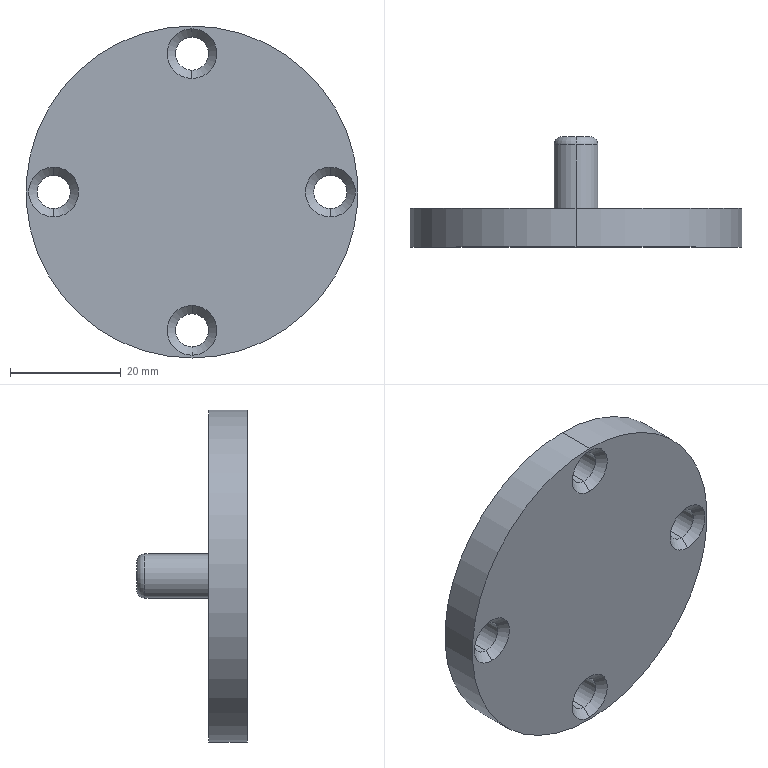Part | SolidWorks | features ICE 2, Extrusion 1, Fillet 1, HoleWzd 1 | 1 solid | 28 faces | box 60 x 20 x 60 mm | volume 17734 mm3 | cylinder 14 | cone 8 | plane 4 | torus 2 | commonest cylinder face diameters 6 x8 8 x2 40 x2 60 x2
STEP:
#1=CARTESIAN_POINT('',(0.,18.5,-4.));
#2=VERTEX_POINT('',#1);
#3=CARTESIAN_POINT('',(0.,18.5,4.));
#4=VERTEX_POINT('',#3);
#5=CARTESIAN_POINT('',(0.,18.5,0.));
#6=DIRECTION('',(0.,-1.,0.));
#7=DIRECTION('',(0.,0.,1.));
#8=AXIS2_PLACEMENT_3D('',#5,#6,#7);
#9=CIRCLE('',#8,4.);
#10=EDGE_CURVE('',#2,#4,#9,.T.);
#11=ORIENTED_EDGE('',*,*,#10,.F.);
#12=CARTESIAN_POINT('',(0.,20.,-2.5));
#13=VERTEX_POINT('',#12);
#14=CARTESIAN_POINT('',(0.,18.5,-2.5));
#15=DIRECTION('',(1.,0.,0.));
#16=DIRECTION('',(0.,0.,-1.));
#17=AXIS2_PLACEMENT_3D('',#14,#15,#16);
#18=CIRCLE('',#17,1.5);
#19=EDGE_CURVE('',#2,#13,#18,.T.);
#20=ORIENTED_EDGE('',*,*,#19,.T.);
#21=CARTESIAN_POINT('',(0.,20.,2.5));
#22=VERTEX_POINT('',#21);
#23=CARTESIAN_POINT('',(0.,20.,0.));
#24=DIRECTION('',(0.,1.,0.));
#25=DIRECTION('',(0.,0.,1.));
#26=AXIS2_PLACEMENT_3D('',#23,#24,#25);
#27=CIRCLE('',#26,2.5);
#28=EDGE_CURVE('',#22,#13,#27,.T.);
#29=ORIENTED_EDGE('',*,*,#28,.F.);
#30=CARTESIAN_POINT('',(0.,18.5,2.5));
#31=DIRECTION('',(-1.,0.,0.));
#32=DIRECTION('',(0.,0.,1.));
#33=AXIS2_PLACEMENT_3D('',#30,#31,#32);
#34=CIRCLE('',#33,1.5);
#35=EDGE_CURVE('',#4,#22,#34,.T.);
#36=ORIENTED_EDGE('',*,*,#35,.F.);
#37=EDGE_LOOP('',(#11,#20,#29,#36));
#38=FACE_OUTER_BOUND('',#37,.T.);
#39=CARTESIAN_POINT('',(0.,18.5,0.));
#40=DIRECTION('',(0.,1.,0.));
#41=DIRECTION('',(0.,0.,1.));
#42=AXIS2_PLACEMENT_3D('',#39,#40,#41);
#43=TOROIDAL_SURFACE('',#42,2.5,1.5);
#44=ADVANCED_FACE('',(#38),#43,.T.);
#45=CARTESIAN_POINT('',(0.,1.5,-22.));
#46=VERTEX_POINT('',#45);
#47=CARTESIAN_POINT('',(0.,1.5,-28.));
#48=VERTEX_POINT('',#47);
#49=CARTESIAN_POINT('',(0.,1.5,-25.));
#50=DIRECTION('',(0.,-1.,0.));
#51=DIRECTION('',(0.,0.,-1.));
#52=AXIS2_PLACEMENT_3D('',#49,#50,#51);
#53=CIRCLE('',#52,3.);
#54=EDGE_CURVE('',#46,#48,#53,.T.);
#55=ORIENTED_EDGE('',*,*,#54,.F.);
#56=CARTESIAN_POINT('',(0.,0.,-20.5));
#57=VERTEX_POINT('',#56);
#58=CARTESIAN_POINT('',(0.,0.,-20.5));
#59=DIRECTION('',(0.,-0.7071,0.7071));
#60=VECTOR('',#59,1000.);
#61=LINE('',#58,#60);
#62=EDGE_CURVE('',#46,#57,#61,.T.);
#63=ORIENTED_EDGE('',*,*,#62,.T.);
#64=CARTESIAN_POINT('',(0.,0.,-29.5));
#65=VERTEX_POINT('',#64);
#66=CARTESIAN_POINT('',(0.,0.,-25.));
#67=DIRECTION('',(0.,-1.,0.));
#68=DIRECTION('',(0.,0.,-1.));
#69=AXIS2_PLACEMENT_3D('',#66,#67,#68);
#70=CIRCLE('',#69,4.5);
#71=EDGE_CURVE('',#57,#65,#70,.T.);
#72=ORIENTED_EDGE('',*,*,#71,.T.);
#73=CARTESIAN_POINT('',(0.,0.,-29.5));
#74=DIRECTION('',(0.,-0.7071,-0.7071));
#75=VECTOR('',#74,1000.);
#76=LINE('',#73,#75);
#77=EDGE_CURVE('',#48,#65,#76,.T.);
#78=ORIENTED_EDGE('',*,*,#77,.F.);
#79=EDGE_LOOP('',(#55,#63,#72,#78));
#80=FACE_OUTER_BOUND('',#79,.T.);
#81=CARTESIAN_POINT('',(0.,0.,-25.));
#82=DIRECTION('',(0.,-1.,0.));
#83=DIRECTION('',(0.,0.,-1.));
#84=AXIS2_PLACEMENT_3D('',#81,#82,#83);
#85=CONICAL_SURFACE('',#84,4.5,0.7854);
#86=ADVANCED_FACE('',(#80),#85,.F.);
#87=CARTESIAN_POINT('',(0.,7.,-28.));
#88=VERTEX_POINT('',#87);
#89=CARTESIAN_POINT('',(0.,7.,-22.));
#90=VERTEX_POINT('',#89);
#91=CARTESIAN_POINT('',(0.,7.,-25.));
#92=DIRECTION('',(0.,1.,0.));
#93=DIRECTION('',(0.,0.,1.));
#94=AXIS2_PLACEMENT_3D('',#91,#92,#93);
#95=CIRCLE('',#94,3.);
#96=EDGE_CURVE('',#88,#90,#95,.T.);
#97=ORIENTED_EDGE('',*,*,#96,.T.);
#98=CARTESIAN_POINT('',(0.,0.,-22.));
#99=DIRECTION('',(0.,-1.,0.));
#100=VECTOR('',#99,1000.);
#101=LINE('',#98,#100);
#102=EDGE_CURVE('',#90,#46,#101,.T.);
#103=ORIENTED_EDGE('',*,*,#102,.T.);
#104=ORIENTED_EDGE('',*,*,#54,.T.);
#105=CARTESIAN_POINT('',(0.,0.,-28.));
#106=DIRECTION('',(0.,-1.,0.));
#107=VECTOR('',#106,1000.);
#108=LINE('',#105,#107);
#109=EDGE_CURVE('',#88,#48,#108,.T.);
#110=ORIENTED_EDGE('',*,*,#109,.F.);
#111=EDGE_LOOP('',(#97,#103,#104,#110));
#112=FACE_OUTER_BOUND('',#111,.T.);
#113=CARTESIAN_POINT('',(0.,0.,-25.));
#114=DIRECTION('',(0.,-1.,0.));
#115=DIRECTION('',(0.,0.,-1.));
#116=AXIS2_PLACEMENT_3D('',#113,#114,#115);
#117=CYLINDRICAL_SURFACE('',#116,3.);
#118=ADVANCED_FACE('',(#112),#117,.F.);
#119=CARTESIAN_POINT('',(-25.,1.5,3.));
#120=VERTEX_POINT('',#119);
#121=CARTESIAN_POINT('',(-25.,1.5,-3.));
#122=VERTEX_POINT('',#121);
#123=CARTESIAN_POINT('',(-25.,1.5,0.));
#124=DIRECTION('',(0.,-1.,0.));
#125=DIRECTION('',(0.,0.,-1.));
#126=AXIS2_PLACEMENT_3D('',#123,#124,#125);
#127=CIRCLE('',#126,3.);
#128=EDGE_CURVE('',#120,#122,#127,.T.);
#129=ORIENTED_EDGE('',*,*,#128,.F.);
#130=CARTESIAN_POINT('',(-25.,0.,4.5));
#131=VERTEX_POINT('',#130);
#132=CARTESIAN_POINT('',(-25.,0.,4.5));
#133=DIRECTION('',(0.,-0.7071,0.7071));
#134=VECTOR('',#133,1000.);
#135=LINE('',#132,#134);
#136=EDGE_CURVE('',#120,#131,#135,.T.);
#137=ORIENTED_EDGE('',*,*,#136,.T.);
#138=CARTESIAN_POINT('',(-25.,0.,-4.5));
#139=VERTEX_POINT('',#138);
#140=CARTESIAN_POINT('',(-25.,0.,0.));
#141=DIRECTION('',(0.,-1.,0.));
#142=DIRECTION('',(0.,0.,-1.));
#143=AXIS2_PLACEMENT_3D('',#140,#141,#142);
#144=CIRCLE('',#143,4.5);
#145=EDGE_CURVE('',#131,#139,#144,.T.);
#146=ORIENTED_EDGE('',*,*,#145,.T.);
#147=CARTESIAN_POINT('',(-25.,0.,-4.5));
#148=DIRECTION('',(0.,-0.7071,-0.7071));
#149=VECTOR('',#148,1000.);
#150=LINE('',#147,#149);
#151=EDGE_CURVE('',#122,#139,#150,.T.);
#152=ORIENTED_EDGE('',*,*,#151,.F.);
#153=EDGE_LOOP('',(#129,#137,#146,#152));
#154=FACE_OUTER_BOUND('',#153,.T.);
#155=CARTESIAN_POINT('',(-25.,0.,0.));
#156=DIRECTION('',(0.,-1.,0.));
#157=DIRECTION('',(0.,0.,-1.));
#158=AXIS2_PLACEMENT_3D('',#155,#156,#157);
#159=CONICAL_SURFACE('',#158,4.5,0.7854);
#160=ADVANCED_FACE('',(#154),#159,.F.);
#161=CARTESIAN_POINT('',(-25.,7.,-3.));
#162=VERTEX_POINT('',#161);
#163=CARTESIAN_POINT('',(-25.,7.,3.));
#164=VERTEX_POINT('',#163);
#165=CARTESIAN_POINT('',(-25.,7.,0.));
#166=DIRECTION('',(0.,1.,0.));
#167=DIRECTION('',(0.,0.,1.));
#168=AXIS2_PLACEMENT_3D('',#165,#166,#167);
#169=CIRCLE('',#168,3.);
#170=EDGE_CURVE('',#162,#164,#169,.T.);
#171=ORIENTED_EDGE('',*,*,#170,.T.);
#172=CARTESIAN_POINT('',(-25.,0.,3.));
#173=DIRECTION('',(0.,-1.,0.));
#174=VECTOR('',#173,1000.);
#175=LINE('',#172,#174);
#176=EDGE_CURVE('',#164,#120,#175,.T.);
#177=ORIENTED_EDGE('',*,*,#176,.T.);
#178=ORIENTED_EDGE('',*,*,#128,.T.);
#179=CARTESIAN_POINT('',(-25.,0.,-3.));
#180=DIRECTION('',(0.,-1.,0.));
#181=VECTOR('',#180,1000.);
#182=LINE('',#179,#181);
#183=EDGE_CURVE('',#162,#122,#182,.T.);
#184=ORIENTED_EDGE('',*,*,#183,.F.);
#185=EDGE_LOOP('',(#171,#177,#178,#184));
#186=FACE_OUTER_BOUND('',#185,.T.);
#187=CARTESIAN_POINT('',(-25.,0.,0.));
#188=DIRECTION('',(0.,-1.,0.));
#189=DIRECTION('',(0.,0.,-1.));
#190=AXIS2_PLACEMENT_3D('',#187,#188,#189);
#191=CYLINDRICAL_SURFACE('',#190,3.);
#192=ADVANCED_FACE('',(#186),#191,.F.);
#193=CARTESIAN_POINT('',(0.,1.5,28.));
#194=VERTEX_POINT('',#193);
#195=CARTESIAN_POINT('',(0.,1.5,22.));
#196=VERTEX_POINT('',#195);
#197=CARTESIAN_POINT('',(0.,1.5,25.));
#198=DIRECTION('',(0.,-1.,0.));
#199=DIRECTION('',(0.,0.,-1.));
#200=AXIS2_PLACEMENT_3D('',#197,#198,#199);
#201=CIRCLE('',#200,3.);
#202=EDGE_CURVE('',#194,#196,#201,.T.);
#203=ORIENTED_EDGE('',*,*,#202,.F.);
#204=CARTESIAN_POINT('',(0.,0.,29.5));
#205=VERTEX_POINT('',#204);
#206=CARTESIAN_POINT('',(0.,0.,29.5));
#207=DIRECTION('',(0.,-0.7071,0.7071));
#208=VECTOR('',#207,1000.);
#209=LINE('',#206,#208);
#210=EDGE_CURVE('',#194,#205,#209,.T.);
#211=ORIENTED_EDGE('',*,*,#210,.T.);
#212=CARTESIAN_POINT('',(0.,0.,20.5));
#213=VERTEX_POINT('',#212);
#214=CARTESIAN_POINT('',(0.,0.,25.));
#215=DIRECTION('',(0.,-1.,0.));
#216=DIRECTION('',(0.,0.,-1.));
#217=AXIS2_PLACEMENT_3D('',#214,#215,#216);
#218=CIRCLE('',#217,4.5);
#219=EDGE_CURVE('',#205,#213,#218,.T.);
#220=ORIENTED_EDGE('',*,*,#219,.T.);
#221=CARTESIAN_POINT('',(0.,0.,20.5));
#222=DIRECTION('',(0.,-0.7071,-0.7071));
#223=VECTOR('',#222,1000.);
#224=LINE('',#221,#223);
#225=EDGE_CURVE('',#196,#213,#224,.T.);
#226=ORIENTED_EDGE('',*,*,#225,.F.);
#227=EDGE_LOOP('',(#203,#211,#220,#226));
#228=FACE_OUTER_BOUND('',#227,.T.);
#229=CARTESIAN_POINT('',(0.,0.,25.));
#230=DIRECTION('',(0.,-1.,0.));
#231=DIRECTION('',(0.,0.,-1.));
#232=AXIS2_PLACEMENT_3D('',#229,#230,#231);
#233=CONICAL_SURFACE('',#232,4.5,0.7854);
#234=ADVANCED_FACE('',(#228),#233,.F.);
#235=CARTESIAN_POINT('',(0.,7.,22.));
#236=VERTEX_POINT('',#235);
#237=CARTESIAN_POINT('',(0.,7.,28.));
#238=VERTEX_POINT('',#237);
#239=CARTESIAN_POINT('',(0.,7.,25.));
#240=DIRECTION('',(0.,1.,0.));
#241=DIRECTION('',(0.,0.,1.));
#242=AXIS2_PLACEMENT_3D('',#239,#240,#241);
#243=CIRCLE('',#242,3.);
#244=EDGE_CURVE('',#236,#238,#243,.T.);
#245=ORIENTED_EDGE('',*,*,#244,.T.);
#246=CARTESIAN_POINT('',(0.,0.,28.));
#247=DIRECTION('',(0.,-1.,0.));
#248=VECTOR('',#247,1000.);
#249=LINE('',#246,#248);
#250=EDGE_CURVE('',#238,#194,#249,.T.);
#251=ORIENTED_EDGE('',*,*,#250,.T.);
#252=ORIENTED_EDGE('',*,*,#202,.T.);
#253=CARTESIAN_POINT('',(0.,0.,22.));
#254=DIRECTION('',(0.,-1.,0.));
#255=VECTOR('',#254,1000.);
#256=LINE('',#253,#255);
#257=EDGE_CURVE('',#236,#196,#256,.T.);
#258=ORIENTED_EDGE('',*,*,#257,.F.);
#259=EDGE_LOOP('',(#245,#251,#252,#258));
#260=FACE_OUTER_BOUND('',#259,.T.);
#261=CARTESIAN_POINT('',(0.,0.,25.));
#262=DIRECTION('',(0.,-1.,0.));
#263=DIRECTION('',(0.,0.,-1.));
#264=AXIS2_PLACEMENT_3D('',#261,#262,#263);
#265=CYLINDRICAL_SURFACE('',#264,3.);
#266=ADVANCED_FACE('',(#260),#265,.F.);
#267=CARTESIAN_POINT('',(25.,1.5,3.));
#268=VERTEX_POINT('',#267);
#269=CARTESIAN_POINT('',(25.,1.5,-3.));
#270=VERTEX_POINT('',#269);
#271=CARTESIAN_POINT('',(25.,1.5,0.));
#272=DIRECTION('',(0.,-1.,0.));
#273=DIRECTION('',(0.,0.,-1.));
#274=AXIS2_PLACEMENT_3D('',#271,#272,#273);
#275=CIRCLE('',#274,3.);
#276=EDGE_CURVE('',#268,#270,#275,.T.);
#277=ORIENTED_EDGE('',*,*,#276,.F.);
#278=CARTESIAN_POINT('',(25.,0.,4.5));
#279=VERTEX_POINT('',#278);
#280=CARTESIAN_POINT('',(25.,0.,4.5));
#281=DIRECTION('',(0.,-0.7071,0.7071));
#282=VECTOR('',#281,1000.);
#283=LINE('',#280,#282);
#284=EDGE_CURVE('',#268,#279,#283,.T.);
#285=ORIENTED_EDGE('',*,*,#284,.T.);
#286=CARTESIAN_POINT('',(25.,0.,-4.5));
#287=VERTEX_POINT('',#286);
#288=CARTESIAN_POINT('',(25.,0.,0.));
#289=DIRECTION('',(0.,-1.,0.));
#290=DIRECTION('',(0.,0.,-1.));
#291=AXIS2_PLACEMENT_3D('',#288,#289,#290);
#292=CIRCLE('',#291,4.5);
#293=EDGE_CURVE('',#279,#287,#292,.T.);
#294=ORIENTED_EDGE('',*,*,#293,.T.);
#295=CARTESIAN_POINT('',(25.,0.,-4.5));
#296=DIRECTION('',(0.,-0.7071,-0.7071));
#297=VECTOR('',#296,1000.);
#298=LINE('',#295,#297);
#299=EDGE_CURVE('',#270,#287,#298,.T.);
#300=ORIENTED_EDGE('',*,*,#299,.F.);
#301=EDGE_LOOP('',(#277,#285,#294,#300));
#302=FACE_OUTER_BOUND('',#301,.T.);
#303=CARTESIAN_POINT('',(25.,0.,0.));
#304=DIRECTION('',(0.,-1.,0.));
#305=DIRECTION('',(0.,0.,-1.));
#306=AXIS2_PLACEMENT_3D('',#303,#304,#305);
#307=CONICAL_SURFACE('',#306,4.5,0.7854);
#308=ADVANCED_FACE('',(#302),#307,.F.);
#309=CARTESIAN_POINT('',(25.,7.,-3.));
#310=VERTEX_POINT('',#309);
#311=CARTESIAN_POINT('',(25.,7.,3.));
#312=VERTEX_POINT('',#311);
#313=CARTESIAN_POINT('',(25.,7.,0.));
#314=DIRECTION('',(0.,1.,0.));
#315=DIRECTION('',(0.,0.,1.));
#316=AXIS2_PLACEMENT_3D('',#313,#314,#315);
#317=CIRCLE('',#316,3.);
#318=EDGE_CURVE('',#310,#312,#317,.T.);
#319=ORIENTED_EDGE('',*,*,#318,.T.);
#320=CARTESIAN_POINT('',(25.,0.,3.));
#321=DIRECTION('',(0.,-1.,0.));
#322=VECTOR('',#321,1000.);
#323=LINE('',#320,#322);
#324=EDGE_CURVE('',#312,#268,#323,.T.);
#325=ORIENTED_EDGE('',*,*,#324,.T.);
#326=ORIENTED_EDGE('',*,*,#276,.T.);
#327=CARTESIAN_POINT('',(25.,0.,-3.));
#328=DIRECTION('',(0.,-1.,0.));
#329=VECTOR('',#328,1000.);
#330=LINE('',#327,#329);
#331=EDGE_CURVE('',#310,#270,#330,.T.);
#332=ORIENTED_EDGE('',*,*,#331,.F.);
#333=EDGE_LOOP('',(#319,#325,#326,#332));
#334=FACE_OUTER_BOUND('',#333,.T.);
#335=CARTESIAN_POINT('',(25.,0.,0.));
#336=DIRECTION('',(0.,-1.,0.));
#337=DIRECTION('',(0.,0.,-1.));
#338=AXIS2_PLACEMENT_3D('',#335,#336,#337);
#339=CYLINDRICAL_SURFACE('',#338,3.);
#340=ADVANCED_FACE('',(#334),#339,.F.);
#341=ORIENTED_EDGE('',*,*,#10,.T.);
#342=CARTESIAN_POINT('',(0.,5.5,4.));
#343=VERTEX_POINT('',#342);
#344=CARTESIAN_POINT('',(0.,20.,4.));
#345=DIRECTION('',(0.,-1.,0.));
#346=VECTOR('',#345,1000.);
#347=LINE('',#344,#346);
#348=EDGE_CURVE('',#4,#343,#347,.T.);
#349=ORIENTED_EDGE('',*,*,#348,.T.);
#350=CARTESIAN_POINT('',(0.,5.5,-4.));
#351=VERTEX_POINT('',#350);
#352=CARTESIAN_POINT('',(0.,5.5,0.));
#353=DIRECTION('',(0.,1.,0.));
#354=DIRECTION('',(0.,0.,1.));
#355=AXIS2_PLACEMENT_3D('',#352,#353,#354);
#356=CIRCLE('',#355,4.);
#357=EDGE_CURVE('',#343,#351,#356,.T.);
#358=ORIENTED_EDGE('',*,*,#357,.T.);
#359=CARTESIAN_POINT('',(0.,20.,-4.));
#360=DIRECTION('',(0.,-1.,0.));
#361=VECTOR('',#360,1000.);
#362=LINE('',#359,#361);
#363=EDGE_CURVE('',#2,#351,#362,.T.);
#364=ORIENTED_EDGE('',*,*,#363,.F.);
#365=EDGE_LOOP('',(#341,#349,#358,#364));
#366=FACE_OUTER_BOUND('',#365,.T.);
#367=CARTESIAN_POINT('',(0.,20.,0.));
#368=DIRECTION('',(0.,-1.,0.));
#369=DIRECTION('',(0.,0.,-1.));
#370=AXIS2_PLACEMENT_3D('',#367,#368,#369);
#371=CYLINDRICAL_SURFACE('',#370,4.);
#372=ADVANCED_FACE('',(#366),#371,.T.);
#373=CARTESIAN_POINT('',(0.,5.5,-20.));
#374=VERTEX_POINT('',#373);
#375=CARTESIAN_POINT('',(0.,5.5,20.));
#376=VERTEX_POINT('',#375);
#377=CARTESIAN_POINT('',(0.,5.5,0.));
#378=DIRECTION('',(0.,1.,0.));
#379=DIRECTION('',(0.,0.,1.));
#380=AXIS2_PLACEMENT_3D('',#377,#378,#379);
#381=CIRCLE('',#380,20.);
#382=EDGE_CURVE('',#374,#376,#381,.T.);
#383=ORIENTED_EDGE('',*,*,#382,.F.);
#384=CARTESIAN_POINT('',(0.,7.,-20.));
#385=VERTEX_POINT('',#384);
#386=CARTESIAN_POINT('',(0.,5.5,-20.));
#387=DIRECTION('',(0.,1.,0.));
#388=VECTOR('',#387,1000.);
#389=LINE('',#386,#388);
#390=EDGE_CURVE('',#374,#385,#389,.T.);
#391=ORIENTED_EDGE('',*,*,#390,.T.);
#392=CARTESIAN_POINT('',(0.,7.,20.));
#393=VERTEX_POINT('',#392);
#394=CARTESIAN_POINT('',(0.,7.,0.));
#395=DIRECTION('',(0.,1.,0.));
#396=DIRECTION('',(0.,0.,1.));
#397=AXIS2_PLACEMENT_3D('',#394,#395,#396);
#398=CIRCLE('',#397,20.);
#399=EDGE_CURVE('',#385,#393,#398,.T.);
#400=ORIENTED_EDGE('',*,*,#399,.T.);
#401=CARTESIAN_POINT('',(0.,5.5,20.));
#402=DIRECTION('',(0.,1.,0.));
#403=VECTOR('',#402,1000.);
#404=LINE('',#401,#403);
#405=EDGE_CURVE('',#376,#393,#404,.T.);
#406=ORIENTED_EDGE('',*,*,#405,.F.);
#407=EDGE_LOOP('',(#383,#391,#400,#406));
#408=FACE_OUTER_BOUND('',#407,.T.);
#409=CARTESIAN_POINT('',(0.,5.5,0.));
#410=DIRECTION('',(0.,1.,0.));
#411=DIRECTION('',(0.,0.,1.));
#412=AXIS2_PLACEMENT_3D('',#409,#410,#411);
#413=CYLINDRICAL_SURFACE('',#412,20.);
#414=ADVANCED_FACE('',(#408),#413,.F.);
#415=CARTESIAN_POINT('',(0.,7.,30.));
#416=VERTEX_POINT('',#415);
#417=CARTESIAN_POINT('',(0.,7.,-30.));
#418=VERTEX_POINT('',#417);
#419=CARTESIAN_POINT('',(0.,7.,0.));
#420=DIRECTION('',(0.,1.,0.));
#421=DIRECTION('',(0.,0.,1.));
#422=AXIS2_PLACEMENT_3D('',#419,#420,#421);
#423=CIRCLE('',#422,30.);
#424=EDGE_CURVE('',#416,#418,#423,.T.);
#425=ORIENTED_EDGE('',*,*,#424,.F.);
#426=CARTESIAN_POINT('',(0.,0.,30.));
#427=VERTEX_POINT('',#426);
#428=CARTESIAN_POINT('',(0.,7.,30.));
#429=DIRECTION('',(0.,-1.,0.));
#430=VECTOR('',#429,1000.);
#431=LINE('',#428,#430);
#432=EDGE_CURVE('',#416,#427,#431,.T.);
#433=ORIENTED_EDGE('',*,*,#432,.T.);
#434=CARTESIAN_POINT('',(0.,0.,-30.));
#435=VERTEX_POINT('',#434);
#436=CARTESIAN_POINT('',(0.,0.,0.));
#437=DIRECTION('',(0.,1.,0.));
#438=DIRECTION('',(0.,0.,1.));
#439=AXIS2_PLACEMENT_3D('',#436,#437,#438);
#440=CIRCLE('',#439,30.);
#441=EDGE_CURVE('',#427,#435,#440,.T.);
#442=ORIENTED_EDGE('',*,*,#441,.T.);
#443=CARTESIAN_POINT('',(0.,7.,-30.));
#444=DIRECTION('',(0.,-1.,0.));
#445=VECTOR('',#444,1000.);
#446=LINE('',#443,#445);
#447=EDGE_CURVE('',#418,#435,#446,.T.);
#448=ORIENTED_EDGE('',*,*,#447,.F.);
#449=EDGE_LOOP('',(#425,#433,#442,#448));
#450=FACE_OUTER_BOUND('',#449,.T.);
#451=CARTESIAN_POINT('',(0.,7.,0.));
#452=DIRECTION('',(0.,-1.,0.));
#453=DIRECTION('',(0.,0.,-1.));
#454=AXIS2_PLACEMENT_3D('',#451,#452,#453);
#455=CYLINDRICAL_SURFACE('',#454,30.);
#456=ADVANCED_FACE('',(#450),#455,.T.);
#457=ORIENTED_EDGE('',*,*,#432,.F.);
#458=CARTESIAN_POINT('',(0.,7.,0.));
#459=DIRECTION('',(0.,1.,0.));
#460=DIRECTION('',(0.,0.,1.));
#461=AXIS2_PLACEMENT_3D('',#458,#459,#460);
#462=CIRCLE('',#461,30.);
#463=EDGE_CURVE('',#418,#416,#462,.T.);
#464=ORIENTED_EDGE('',*,*,#463,.F.);
#465=ORIENTED_EDGE('',*,*,#447,.T.);
#466=CARTESIAN_POINT('',(0.,0.,0.));
#467=DIRECTION('',(0.,1.,0.));
#468=DIRECTION('',(0.,0.,1.));
#469=AXIS2_PLACEMENT_3D('',#466,#467,#468);
#470=CIRCLE('',#469,30.);
#471=EDGE_CURVE('',#435,#427,#470,.T.);
#472=ORIENTED_EDGE('',*,*,#471,.T.);
#473=EDGE_LOOP('',(#457,#464,#465,#472));
#474=FACE_OUTER_BOUND('',#473,.T.);
#475=CARTESIAN_POINT('',(0.,7.,0.));
#476=DIRECTION('',(0.,-1.,0.));
#477=DIRECTION('',(0.,0.,-1.));
#478=AXIS2_PLACEMENT_3D('',#475,#476,#477);
#479=CYLINDRICAL_SURFACE('',#478,30.);
#480=ADVANCED_FACE('',(#474),#479,.T.);
#481=ORIENTED_EDGE('',*,*,#96,.F.);
#482=CARTESIAN_POINT('',(0.,7.,-25.));
#483=DIRECTION('',(0.,1.,0.));
#484=DIRECTION('',(0.,0.,1.));
#485=AXIS2_PLACEMENT_3D('',#482,#483,#484);
#486=CIRCLE('',#485,3.);
#487=EDGE_CURVE('',#90,#88,#486,.T.);
#488=ORIENTED_EDGE('',*,*,#487,.F.);
#489=EDGE_LOOP('',(#481,#488));
#490=FACE_BOUND('',#489,.T.);
#491=ORIENTED_EDGE('',*,*,#170,.F.);
#492=CARTESIAN_POINT('',(-25.,7.,0.));
#493=DIRECTION('',(0.,1.,0.));
#494=DIRECTION('',(0.,0.,1.));
#495=AXIS2_PLACEMENT_3D('',#492,#493,#494);
#496=CIRCLE('',#495,3.);
#497=EDGE_CURVE('',#164,#162,#496,.T.);
#498=ORIENTED_EDGE('',*,*,#497,.F.);
#499=EDGE_LOOP('',(#491,#498));
#500=FACE_BOUND('',#499,.T.);
#501=ORIENTED_EDGE('',*,*,#244,.F.);
#502=CARTESIAN_POINT('',(0.,7.,25.));
#503=DIRECTION('',(0.,1.,0.));
#504=DIRECTION('',(0.,0.,1.));
#505=AXIS2_PLACEMENT_3D('',#502,#503,#504);
#506=CIRCLE('',#505,3.);
#507=EDGE_CURVE('',#238,#236,#506,.T.);
#508=ORIENTED_EDGE('',*,*,#507,.F.);
#509=EDGE_LOOP('',(#501,#508));
#510=FACE_BOUND('',#509,.T.);
#511=ORIENTED_EDGE('',*,*,#318,.F.);
#512=CARTESIAN_POINT('',(25.,7.,0.));
#513=DIRECTION('',(0.,1.,0.));
#514=DIRECTION('',(0.,0.,1.));
#515=AXIS2_PLACEMENT_3D('',#512,#513,#514);
#516=CIRCLE('',#515,3.);
#517=EDGE_CURVE('',#312,#310,#516,.T.);
#518=ORIENTED_EDGE('',*,*,#517,.F.);
#519=EDGE_LOOP('',(#511,#518));
#520=FACE_BOUND('',#519,.T.);
#521=CARTESIAN_POINT('',(0.,7.,0.));
#522=DIRECTION('',(0.,1.,0.));
#523=DIRECTION('',(0.,0.,1.));
#524=AXIS2_PLACEMENT_3D('',#521,#522,#523);
#525=CIRCLE('',#524,20.);
#526=EDGE_CURVE('',#393,#385,#525,.T.);
#527=ORIENTED_EDGE('',*,*,#526,.F.);
#528=ORIENTED_EDGE('',*,*,#399,.F.);
#529=EDGE_LOOP('',(#527,#528));
#530=FACE_BOUND('',#529,.T.);
#531=ORIENTED_EDGE('',*,*,#463,.T.);
#532=ORIENTED_EDGE('',*,*,#424,.T.);
#533=EDGE_LOOP('',(#531,#532));
#534=FACE_OUTER_BOUND('',#533,.T.);
#535=CARTESIAN_POINT('',(0.,7.,0.));
#536=DIRECTION('',(0.,1.,0.));
#537=DIRECTION('',(0.,0.,1.));
#538=AXIS2_PLACEMENT_3D('',#535,#536,#537);
#539=PLANE('',#538);
#540=ADVANCED_FACE('',(#490,#500,#510,#520,#530,#534),#539,.T.);
#541=CARTESIAN_POINT('',(0.,0.,-25.));
#542=DIRECTION('',(0.,-1.,0.));
#543=DIRECTION('',(0.,0.,-1.));
#544=AXIS2_PLACEMENT_3D('',#541,#542,#543);
#545=CIRCLE('',#544,4.5);
#546=EDGE_CURVE('',#65,#57,#545,.T.);
#547=ORIENTED_EDGE('',*,*,#546,.F.);
#548=ORIENTED_EDGE('',*,*,#71,.F.);
#549=EDGE_LOOP('',(#547,#548));
#550=FACE_BOUND('',#549,.T.);
#551=CARTESIAN_POINT('',(-25.,0.,0.));
#552=DIRECTION('',(0.,-1.,0.));
#553=DIRECTION('',(0.,0.,-1.));
#554=AXIS2_PLACEMENT_3D('',#551,#552,#553);
#555=CIRCLE('',#554,4.5);
#556=EDGE_CURVE('',#139,#131,#555,.T.);
#557=ORIENTED_EDGE('',*,*,#556,.F.);
#558=ORIENTED_EDGE('',*,*,#145,.F.);
#559=EDGE_LOOP('',(#557,#558));
#560=FACE_BOUND('',#559,.T.);
#561=CARTESIAN_POINT('',(0.,0.,25.));
#562=DIRECTION('',(0.,-1.,0.));
#563=DIRECTION('',(0.,0.,-1.));
#564=AXIS2_PLACEMENT_3D('',#561,#562,#563);
#565=CIRCLE('',#564,4.5);
#566=EDGE_CURVE('',#213,#205,#565,.T.);
#567=ORIENTED_EDGE('',*,*,#566,.F.);
#568=ORIENTED_EDGE('',*,*,#219,.F.);
#569=EDGE_LOOP('',(#567,#568));
#570=FACE_BOUND('',#569,.T.);
#571=CARTESIAN_POINT('',(25.,0.,0.));
#572=DIRECTION('',(0.,-1.,0.));
#573=DIRECTION('',(0.,0.,-1.));
#574=AXIS2_PLACEMENT_3D('',#571,#572,#573);
#575=CIRCLE('',#574,4.5);
#576=EDGE_CURVE('',#287,#279,#575,.T.);
#577=ORIENTED_EDGE('',*,*,#576,.F.);
#578=ORIENTED_EDGE('',*,*,#293,.F.);
#579=EDGE_LOOP('',(#577,#578));
#580=FACE_BOUND('',#579,.T.);
#581=ORIENTED_EDGE('',*,*,#471,.F.);
#582=ORIENTED_EDGE('',*,*,#441,.F.);
#583=EDGE_LOOP('',(#581,#582));
#584=FACE_OUTER_BOUND('',#583,.T.);
#585=CARTESIAN_POINT('',(0.,0.,0.));
#586=DIRECTION('',(0.,1.,0.));
#587=DIRECTION('',(0.,0.,1.));
#588=AXIS2_PLACEMENT_3D('',#585,#586,#587);
#589=PLANE('',#588);
#590=ADVANCED_FACE('',(#550,#560,#570,#580,#584),#589,.F.);
#591=ORIENTED_EDGE('',*,*,#390,.F.);
#592=CARTESIAN_POINT('',(0.,5.5,0.));
#593=DIRECTION('',(0.,1.,0.));
#594=DIRECTION('',(0.,0.,1.));
#595=AXIS2_PLACEMENT_3D('',#592,#593,#594);
#596=CIRCLE('',#595,20.);
#597=EDGE_CURVE('',#376,#374,#596,.T.);
#598=ORIENTED_EDGE('',*,*,#597,.F.);
#599=ORIENTED_EDGE('',*,*,#405,.T.);
#600=ORIENTED_EDGE('',*,*,#526,.T.);
#601=EDGE_LOOP('',(#591,#598,#599,#600));
#602=FACE_OUTER_BOUND('',#601,.T.);
#603=CARTESIAN_POINT('',(0.,5.5,0.));
#604=DIRECTION('',(0.,1.,0.));
#605=DIRECTION('',(0.,0.,1.));
#606=AXIS2_PLACEMENT_3D('',#603,#604,#605);
#607=CYLINDRICAL_SURFACE('',#606,20.);
#608=ADVANCED_FACE('',(#602),#607,.F.);
#609=CARTESIAN_POINT('',(0.,5.5,0.));
#610=DIRECTION('',(0.,1.,0.));
#611=DIRECTION('',(0.,0.,1.));
#612=AXIS2_PLACEMENT_3D('',#609,#610,#611);
#613=CIRCLE('',#612,4.);
#614=EDGE_CURVE('',#351,#343,#613,.T.);
#615=ORIENTED_EDGE('',*,*,#614,.F.);
#616=ORIENTED_EDGE('',*,*,#357,.F.);
#617=EDGE_LOOP('',(#615,#616));
#618=FACE_BOUND('',#617,.T.);
#619=ORIENTED_EDGE('',*,*,#597,.T.);
#620=ORIENTED_EDGE('',*,*,#382,.T.);
#621=EDGE_LOOP('',(#619,#620));
#622=FACE_OUTER_BOUND('',#621,.T.);
#623=CARTESIAN_POINT('',(0.,5.5,0.));
#624=DIRECTION('',(0.,1.,0.));
#625=DIRECTION('',(0.,0.,1.));
#626=AXIS2_PLACEMENT_3D('',#623,#624,#625);
#627=PLANE('',#626);
#628=ADVANCED_FACE('',(#618,#622),#627,.T.);
#629=ORIENTED_EDGE('',*,*,#28,.T.);
#630=CARTESIAN_POINT('',(0.,20.,0.));
#631=DIRECTION('',(0.,1.,0.));
#632=DIRECTION('',(0.,0.,1.));
#633=AXIS2_PLACEMENT_3D('',#630,#631,#632);
#634=CIRCLE('',#633,2.5);
#635=EDGE_CURVE('',#13,#22,#634,.T.);
#636=ORIENTED_EDGE('',*,*,#635,.T.);
#637=EDGE_LOOP('',(#629,#636));
#638=FACE_OUTER_BOUND('',#637,.T.);
#639=CARTESIAN_POINT('',(0.,20.,0.));
#640=DIRECTION('',(0.,1.,0.));
#641=DIRECTION('',(0.,0.,1.));
#642=AXIS2_PLACEMENT_3D('',#639,#640,#641);
#643=PLANE('',#642);
#644=ADVANCED_FACE('',(#638),#643,.T.);
#645=ORIENTED_EDGE('',*,*,#348,.F.);
#646=CARTESIAN_POINT('',(0.,18.5,0.));
#647=DIRECTION('',(0.,-1.,0.));
#648=DIRECTION('',(0.,0.,1.));
#649=AXIS2_PLACEMENT_3D('',#646,#647,#648);
#650=CIRCLE('',#649,4.);
#651=EDGE_CURVE('',#4,#2,#650,.T.);
#652=ORIENTED_EDGE('',*,*,#651,.T.);
#653=ORIENTED_EDGE('',*,*,#363,.T.);
#654=ORIENTED_EDGE('',*,*,#614,.T.);
#655=EDGE_LOOP('',(#645,#652,#653,#654));
#656=FACE_OUTER_BOUND('',#655,.T.);
#657=CARTESIAN_POINT('',(0.,20.,0.));
#658=DIRECTION('',(0.,-1.,0.));
#659=DIRECTION('',(0.,0.,-1.));
#660=AXIS2_PLACEMENT_3D('',#657,#658,#659);
#661=CYLINDRICAL_SURFACE('',#660,4.);
#662=ADVANCED_FACE('',(#656),#661,.T.);
#663=ORIENTED_EDGE('',*,*,#324,.F.);
#664=ORIENTED_EDGE('',*,*,#517,.T.);
#665=ORIENTED_EDGE('',*,*,#331,.T.);
#666=CARTESIAN_POINT('',(25.,1.5,0.));
#667=DIRECTION('',(0.,-1.,0.));
#668=DIRECTION('',(0.,0.,-1.));
#669=AXIS2_PLACEMENT_3D('',#666,#667,#668);
#670=CIRCLE('',#669,3.);
#671=EDGE_CURVE('',#270,#268,#670,.T.);
#672=ORIENTED_EDGE('',*,*,#671,.T.);
#673=EDGE_LOOP('',(#663,#664,#665,#672));
#674=FACE_OUTER_BOUND('',#673,.T.);
#675=CARTESIAN_POINT('',(25.,0.,0.));
#676=DIRECTION('',(0.,-1.,0.));
#677=DIRECTION('',(0.,0.,-1.));
#678=AXIS2_PLACEMENT_3D('',#675,#676,#677);
#679=CYLINDRICAL_SURFACE('',#678,3.);
#680=ADVANCED_FACE('',(#674),#679,.F.);
#681=ORIENTED_EDGE('',*,*,#284,.F.);
#682=ORIENTED_EDGE('',*,*,#671,.F.);
#683=ORIENTED_EDGE('',*,*,#299,.T.);
#684=ORIENTED_EDGE('',*,*,#576,.T.);
#685=EDGE_LOOP('',(#681,#682,#683,#684));
#686=FACE_OUTER_BOUND('',#685,.T.);
#687=CARTESIAN_POINT('',(25.,0.,0.));
#688=DIRECTION('',(0.,-1.,0.));
#689=DIRECTION('',(0.,0.,-1.));
#690=AXIS2_PLACEMENT_3D('',#687,#688,#689);
#691=CONICAL_SURFACE('',#690,4.5,0.7854);
#692=ADVANCED_FACE('',(#686),#691,.F.);
#693=ORIENTED_EDGE('',*,*,#250,.F.);
#694=ORIENTED_EDGE('',*,*,#507,.T.);
#695=ORIENTED_EDGE('',*,*,#257,.T.);
#696=CARTESIAN_POINT('',(0.,1.5,25.));
#697=DIRECTION('',(0.,-1.,0.));
#698=DIRECTION('',(0.,0.,-1.));
#699=AXIS2_PLACEMENT_3D('',#696,#697,#698);
#700=CIRCLE('',#699,3.);
#701=EDGE_CURVE('',#196,#194,#700,.T.);
#702=ORIENTED_EDGE('',*,*,#701,.T.);
#703=EDGE_LOOP('',(#693,#694,#695,#702));
#704=FACE_OUTER_BOUND('',#703,.T.);
#705=CARTESIAN_POINT('',(0.,0.,25.));
#706=DIRECTION('',(0.,-1.,0.));
#707=DIRECTION('',(0.,0.,-1.));
#708=AXIS2_PLACEMENT_3D('',#705,#706,#707);
#709=CYLINDRICAL_SURFACE('',#708,3.);
#710=ADVANCED_FACE('',(#704),#709,.F.);
#711=ORIENTED_EDGE('',*,*,#210,.F.);
#712=ORIENTED_EDGE('',*,*,#701,.F.);
#713=ORIENTED_EDGE('',*,*,#225,.T.);
#714=ORIENTED_EDGE('',*,*,#566,.T.);
#715=EDGE_LOOP('',(#711,#712,#713,#714));
#716=FACE_OUTER_BOUND('',#715,.T.);
#717=CARTESIAN_POINT('',(0.,0.,25.));
#718=DIRECTION('',(0.,-1.,0.));
#719=DIRECTION('',(0.,0.,-1.));
#720=AXIS2_PLACEMENT_3D('',#717,#718,#719);
#721=CONICAL_SURFACE('',#720,4.5,0.7854);
#722=ADVANCED_FACE('',(#716),#721,.F.);
#723=ORIENTED_EDGE('',*,*,#176,.F.);
#724=ORIENTED_EDGE('',*,*,#497,.T.);
#725=ORIENTED_EDGE('',*,*,#183,.T.);
#726=CARTESIAN_POINT('',(-25.,1.5,0.));
#727=DIRECTION('',(0.,-1.,0.));
#728=DIRECTION('',(0.,0.,-1.));
#729=AXIS2_PLACEMENT_3D('',#726,#727,#728);
#730=CIRCLE('',#729,3.);
#731=EDGE_CURVE('',#122,#120,#730,.T.);
#732=ORIENTED_EDGE('',*,*,#731,.T.);
#733=EDGE_LOOP('',(#723,#724,#725,#732));
#734=FACE_OUTER_BOUND('',#733,.T.);
#735=CARTESIAN_POINT('',(-25.,0.,0.));
#736=DIRECTION('',(0.,-1.,0.));
#737=DIRECTION('',(0.,0.,-1.));
#738=AXIS2_PLACEMENT_3D('',#735,#736,#737);
#739=CYLINDRICAL_SURFACE('',#738,3.);
#740=ADVANCED_FACE('',(#734),#739,.F.);
#741=ORIENTED_EDGE('',*,*,#136,.F.);
#742=ORIENTED_EDGE('',*,*,#731,.F.);
#743=ORIENTED_EDGE('',*,*,#151,.T.);
#744=ORIENTED_EDGE('',*,*,#556,.T.);
#745=EDGE_LOOP('',(#741,#742,#743,#744));
#746=FACE_OUTER_BOUND('',#745,.T.);
#747=CARTESIAN_POINT('',(-25.,0.,0.));
#748=DIRECTION('',(0.,-1.,0.));
#749=DIRECTION('',(0.,0.,-1.));
#750=AXIS2_PLACEMENT_3D('',#747,#748,#749);
#751=CONICAL_SURFACE('',#750,4.5,0.7854);
#752=ADVANCED_FACE('',(#746),#751,.F.);
#753=ORIENTED_EDGE('',*,*,#102,.F.);
#754=ORIENTED_EDGE('',*,*,#487,.T.);
#755=ORIENTED_EDGE('',*,*,#109,.T.);
#756=CARTESIAN_POINT('',(0.,1.5,-25.));
#757=DIRECTION('',(0.,-1.,0.));
#758=DIRECTION('',(0.,0.,-1.));
#759=AXIS2_PLACEMENT_3D('',#756,#757,#758);
#760=CIRCLE('',#759,3.);
#761=EDGE_CURVE('',#48,#46,#760,.T.);
#762=ORIENTED_EDGE('',*,*,#761,.T.);
#763=EDGE_LOOP('',(#753,#754,#755,#762));
#764=FACE_OUTER_BOUND('',#763,.T.);
#765=CARTESIAN_POINT('',(0.,0.,-25.));
#766=DIRECTION('',(0.,-1.,0.));
#767=DIRECTION('',(0.,0.,-1.));
#768=AXIS2_PLACEMENT_3D('',#765,#766,#767);
#769=CYLINDRICAL_SURFACE('',#768,3.);
#770=ADVANCED_FACE('',(#764),#769,.F.);
#771=ORIENTED_EDGE('',*,*,#62,.F.);
#772=ORIENTED_EDGE('',*,*,#761,.F.);
#773=ORIENTED_EDGE('',*,*,#77,.T.);
#774=ORIENTED_EDGE('',*,*,#546,.T.);
#775=EDGE_LOOP('',(#771,#772,#773,#774));
#776=FACE_OUTER_BOUND('',#775,.T.);
#777=CARTESIAN_POINT('',(0.,0.,-25.));
#778=DIRECTION('',(0.,-1.,0.));
#779=DIRECTION('',(0.,0.,-1.));
#780=AXIS2_PLACEMENT_3D('',#777,#778,#779);
#781=CONICAL_SURFACE('',#780,4.5,0.7854);
#782=ADVANCED_FACE('',(#776),#781,.F.);
#783=ORIENTED_EDGE('',*,*,#19,.F.);
#784=ORIENTED_EDGE('',*,*,#651,.F.);
#785=ORIENTED_EDGE('',*,*,#35,.T.);
#786=ORIENTED_EDGE('',*,*,#635,.F.);
#787=EDGE_LOOP('',(#783,#784,#785,#786));
#788=FACE_OUTER_BOUND('',#787,.T.);
#789=CARTESIAN_POINT('',(0.,18.5,0.));
#790=DIRECTION('',(0.,1.,0.));
#791=DIRECTION('',(0.,0.,1.));
#792=AXIS2_PLACEMENT_3D('',#789,#790,#791);
#793=TOROIDAL_SURFACE('',#792,2.5,1.5);
#794=ADVANCED_FACE('',(#788),#793,.T.);
#795=CLOSED_SHELL('',(#44,#86,#118,#160,#192,#234,#266,#308,#340,#372,#414,#456,#480,#540,#590,#608,#628,#644,#662,#680,#692,#710,#722,#740,#752,#770,#782,#794));
#796=MANIFOLD_SOLID_BREP('',#795);
#797=CARTESIAN_POINT('',(0.,0.,0.));
#798=DIRECTION('',(0.,0.,1.));
#799=DIRECTION('',(1.,0.,0.));
#800=AXIS2_PLACEMENT_3D('',#797,#798,#799);
#801=(LENGTH_UNIT()NAMED_UNIT(*)SI_UNIT(.MILLI.,.METRE.));
#802=UNCERTAINTY_MEASURE_WITH_UNIT(LENGTH_MEASURE(0.00001),#801,'','');
#803=(NAMED_UNIT(*)PLANE_ANGLE_UNIT()SI_UNIT($,.RADIAN.));
#804=(NAMED_UNIT(*)SI_UNIT($,.STERADIAN.)SOLID_ANGLE_UNIT());
#805=(GEOMETRIC_REPRESENTATION_CONTEXT(3)GLOBAL_UNCERTAINTY_ASSIGNED_CONTEXT((#802))GLOBAL_UNIT_ASSIGNED_CONTEXT((#801,#803,#804))REPRESENTATION_CONTEXT('',''));
#806=ADVANCED_BREP_SHAPE_REPRESENTATION('',(#796,#800),#805);